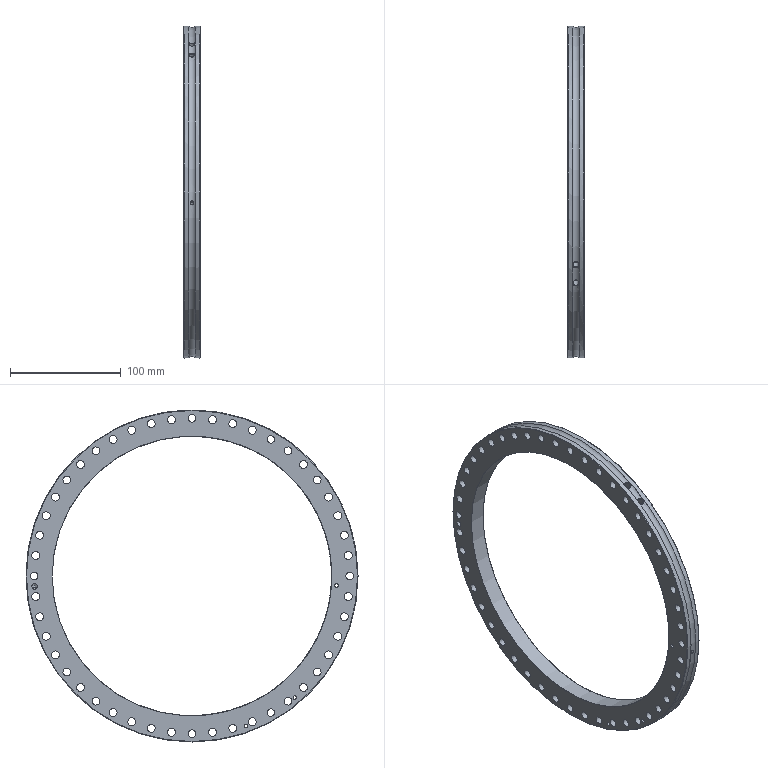Part | STEP file | Part [17] | 1 solid | 77 faces | box 15 x 300 x 300 mm | volume 273448 mm3 | cylinder 62 | cone 6 | torus 5 | plane 4 | commonest cylinder face diameters 7.1 x45 3.5 x4 6.647 x3 3.242 x2 4.917 x2 6 x2